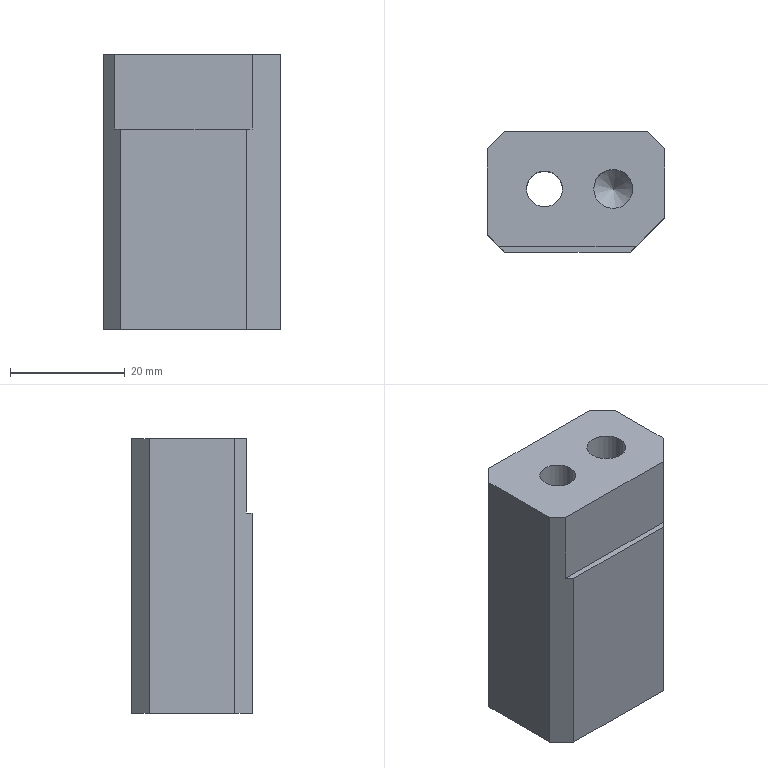Part | NX | features LIN_SOLID_COLOR 2 | 1 solid | 15 faces | box 31 x 21 x 48 mm | volume 26979 mm3 | plane 12 | cylinder 2 | cone 1 | commonest cylinder face diameters 6.28 x1 6.8 x1
STEP:
#1=CARTESIAN_POINT('',(657.878,13.865,1.5));
#2=VERTEX_POINT('',#1);
#3=CARTESIAN_POINT('',(655.878,15.865,1.5));
#4=VERTEX_POINT('',#3);
#5=CARTESIAN_POINT('',(655.878,15.865,1.5));
#6=DIRECTION('',(0.7071,-0.7071,0.));
#7=VECTOR('',#6,1000.);
#8=LINE('',#5,#7);
#9=EDGE_CURVE('',#2,#4,#8,.F.);
#10=ORIENTED_EDGE('',*,*,#9,.F.);
#11=CARTESIAN_POINT('',(681.878,13.865,1.5));
#12=VERTEX_POINT('',#11);
#13=CARTESIAN_POINT('',(305.33,13.865,1.5));
#14=DIRECTION('',(-1.,0.,0.));
#15=VECTOR('',#14,1000.);
#16=LINE('',#13,#15);
#17=EDGE_CURVE('',#12,#2,#16,.T.);
#18=ORIENTED_EDGE('',*,*,#17,.F.);
#19=CARTESIAN_POINT('',(686.878,18.865,1.5));
#20=VERTEX_POINT('',#19);
#21=CARTESIAN_POINT('',(686.878,18.865,1.5));
#22=DIRECTION('',(0.7071,0.7071,0.));
#23=VECTOR('',#22,1000.);
#24=LINE('',#21,#23);
#25=EDGE_CURVE('',#20,#12,#24,.F.);
#26=ORIENTED_EDGE('',*,*,#25,.F.);
#27=CARTESIAN_POINT('',(686.878,30.865,1.5));
#28=VERTEX_POINT('',#27);
#29=CARTESIAN_POINT('',(686.878,23.865,1.5));
#30=DIRECTION('',(0.,-1.,0.));
#31=VECTOR('',#30,1000.);
#32=LINE('',#29,#31);
#33=EDGE_CURVE('',#28,#20,#32,.T.);
#34=ORIENTED_EDGE('',*,*,#33,.F.);
#35=CARTESIAN_POINT('',(683.878,33.865,1.5));
#36=VERTEX_POINT('',#35);
#37=CARTESIAN_POINT('',(683.878,33.865,1.5));
#38=DIRECTION('',(-0.7071,0.7071,0.));
#39=VECTOR('',#38,1000.);
#40=LINE('',#37,#39);
#41=EDGE_CURVE('',#36,#28,#40,.F.);
#42=ORIENTED_EDGE('',*,*,#41,.F.);
#43=CARTESIAN_POINT('',(658.878,33.865,1.5));
#44=VERTEX_POINT('',#43);
#45=CARTESIAN_POINT('',(672.878,33.865,1.5));
#46=DIRECTION('',(1.,0.,0.));
#47=VECTOR('',#46,1000.);
#48=LINE('',#45,#47);
#49=EDGE_CURVE('',#44,#36,#48,.T.);
#50=ORIENTED_EDGE('',*,*,#49,.F.);
#51=CARTESIAN_POINT('',(655.878,30.865,1.5));
#52=VERTEX_POINT('',#51);
#53=CARTESIAN_POINT('',(658.878,33.865,1.5));
#54=DIRECTION('',(-0.7071,-0.7071,0.));
#55=VECTOR('',#54,1000.);
#56=LINE('',#53,#55);
#57=EDGE_CURVE('',#52,#44,#56,.F.);
#58=ORIENTED_EDGE('',*,*,#57,.F.);
#59=CARTESIAN_POINT('',(655.878,23.865,1.5));
#60=DIRECTION('',(0.,1.,0.));
#61=VECTOR('',#60,1000.);
#62=LINE('',#59,#61);
#63=EDGE_CURVE('',#4,#52,#62,.T.);
#64=ORIENTED_EDGE('',*,*,#63,.F.);
#65=EDGE_LOOP('',(#10,#18,#26,#34,#42,#50,#58,#64));
#66=FACE_BOUND('',#65,.T.);
#67=CARTESIAN_POINT('',(669.018,23.865,1.5));
#68=VERTEX_POINT('',#67);
#69=CARTESIAN_POINT('',(665.878,23.865,1.5));
#70=DIRECTION('',(0.,0.,1.));
#71=DIRECTION('',(1.,0.,0.));
#72=AXIS2_PLACEMENT_3D('',#69,#70,#71);
#73=CIRCLE('',#72,3.14);
#74=EDGE_CURVE('',#68,#68,#73,.F.);
#75=ORIENTED_EDGE('',*,*,#74,.T.);
#76=EDGE_LOOP('',(#75));
#77=FACE_BOUND('',#76,.T.);
#78=CARTESIAN_POINT('',(681.278,23.865,1.5));
#79=VERTEX_POINT('',#78);
#80=CARTESIAN_POINT('',(677.878,23.865,1.5));
#81=DIRECTION('',(0.,0.,-1.));
#82=DIRECTION('',(1.,0.,0.));
#83=AXIS2_PLACEMENT_3D('',#80,#81,#82);
#84=CIRCLE('',#83,3.4);
#85=EDGE_CURVE('',#79,#79,#84,.T.);
#86=ORIENTED_EDGE('',*,*,#85,.T.);
#87=EDGE_LOOP('',(#86));
#88=FACE_BOUND('',#87,.T.);
#89=CARTESIAN_POINT('',(305.33,343.366,1.5));
#90=DIRECTION('',(0.,0.,1.));
#91=DIRECTION('',(0.,-1.,0.));
#92=AXIS2_PLACEMENT_3D('',#89,#90,#91);
#93=PLANE('',#92);
#94=ADVANCED_FACE('',(#66,#77,#88),#93,.T.);
#95=CARTESIAN_POINT('',(658.878,12.865,-11.5));
#96=VERTEX_POINT('',#95);
#97=CARTESIAN_POINT('',(680.878,12.865,-11.5));
#98=VERTEX_POINT('',#97);
#99=CARTESIAN_POINT('',(672.878,12.865,-11.5));
#100=DIRECTION('',(1.,0.,0.));
#101=VECTOR('',#100,1000.);
#102=LINE('',#99,#101);
#103=EDGE_CURVE('',#96,#98,#102,.T.);
#104=ORIENTED_EDGE('',*,*,#103,.F.);
#105=CARTESIAN_POINT('',(658.878,12.865,-46.5));
#106=VERTEX_POINT('',#105);
#107=CARTESIAN_POINT('',(658.878,12.865,-28.49));
#108=DIRECTION('',(0.,0.,-1.));
#109=VECTOR('',#108,1000.);
#110=LINE('',#107,#109);
#111=EDGE_CURVE('',#96,#106,#110,.T.);
#112=ORIENTED_EDGE('',*,*,#111,.T.);
#113=CARTESIAN_POINT('',(680.878,12.865,-46.5));
#114=VERTEX_POINT('',#113);
#115=CARTESIAN_POINT('',(672.878,12.865,-46.5));
#116=DIRECTION('',(1.,0.,0.));
#117=VECTOR('',#116,1000.);
#118=LINE('',#115,#117);
#119=EDGE_CURVE('',#106,#114,#118,.T.);
#120=ORIENTED_EDGE('',*,*,#119,.T.);
#121=CARTESIAN_POINT('',(680.878,12.865,-28.49));
#122=DIRECTION('',(0.,0.,1.));
#123=VECTOR('',#122,1000.);
#124=LINE('',#121,#123);
#125=EDGE_CURVE('',#114,#98,#124,.T.);
#126=ORIENTED_EDGE('',*,*,#125,.T.);
#127=EDGE_LOOP('',(#104,#112,#120,#126));
#128=FACE_BOUND('',#127,.T.);
#129=CARTESIAN_POINT('',(672.878,12.865,-28.49));
#130=DIRECTION('',(0.,-1.,0.));
#131=DIRECTION('',(0.,0.,-1.));
#132=AXIS2_PLACEMENT_3D('',#129,#130,#131);
#133=PLANE('',#132);
#134=ADVANCED_FACE('',(#128),#133,.T.);
#135=CARTESIAN_POINT('',(655.878,15.865,-46.5));
#136=VERTEX_POINT('',#135);
#137=CARTESIAN_POINT('',(655.878,15.865,-28.49));
#138=DIRECTION('',(0.,0.,1.));
#139=VECTOR('',#138,1000.);
#140=LINE('',#137,#139);
#141=EDGE_CURVE('',#136,#4,#140,.T.);
#142=ORIENTED_EDGE('',*,*,#141,.T.);
#143=ORIENTED_EDGE('',*,*,#63,.T.);
#144=CARTESIAN_POINT('',(655.878,30.865,-46.5));
#145=VERTEX_POINT('',#144);
#146=CARTESIAN_POINT('',(655.878,30.865,-28.49));
#147=DIRECTION('',(0.,0.,-1.));
#148=VECTOR('',#147,1000.);
#149=LINE('',#146,#148);
#150=EDGE_CURVE('',#52,#145,#149,.T.);
#151=ORIENTED_EDGE('',*,*,#150,.T.);
#152=CARTESIAN_POINT('',(655.878,23.865,-46.5));
#153=DIRECTION('',(0.,-1.,0.));
#154=VECTOR('',#153,1000.);
#155=LINE('',#152,#154);
#156=EDGE_CURVE('',#145,#136,#155,.T.);
#157=ORIENTED_EDGE('',*,*,#156,.T.);
#158=EDGE_LOOP('',(#142,#143,#151,#157));
#159=FACE_BOUND('',#158,.T.);
#160=CARTESIAN_POINT('',(655.878,23.865,-28.49));
#161=DIRECTION('',(-1.,0.,0.));
#162=DIRECTION('',(0.,0.,1.));
#163=AXIS2_PLACEMENT_3D('',#160,#161,#162);
#164=PLANE('',#163);
#165=ADVANCED_FACE('',(#159),#164,.T.);
#166=ORIENTED_EDGE('',*,*,#49,.T.);
#167=CARTESIAN_POINT('',(683.878,33.865,-46.5));
#168=VERTEX_POINT('',#167);
#169=CARTESIAN_POINT('',(683.878,33.865,-28.49));
#170=DIRECTION('',(0.,0.,-1.));
#171=VECTOR('',#170,1000.);
#172=LINE('',#169,#171);
#173=EDGE_CURVE('',#36,#168,#172,.T.);
#174=ORIENTED_EDGE('',*,*,#173,.T.);
#175=CARTESIAN_POINT('',(658.878,33.865,-46.5));
#176=VERTEX_POINT('',#175);
#177=CARTESIAN_POINT('',(672.878,33.865,-46.5));
#178=DIRECTION('',(-1.,0.,0.));
#179=VECTOR('',#178,1000.);
#180=LINE('',#177,#179);
#181=EDGE_CURVE('',#168,#176,#180,.T.);
#182=ORIENTED_EDGE('',*,*,#181,.T.);
#183=CARTESIAN_POINT('',(658.878,33.865,-28.49));
#184=DIRECTION('',(0.,0.,1.));
#185=VECTOR('',#184,1000.);
#186=LINE('',#183,#185);
#187=EDGE_CURVE('',#176,#44,#186,.T.);
#188=ORIENTED_EDGE('',*,*,#187,.T.);
#189=EDGE_LOOP('',(#166,#174,#182,#188));
#190=FACE_BOUND('',#189,.T.);
#191=CARTESIAN_POINT('',(672.878,33.865,-28.49));
#192=DIRECTION('',(0.,1.,0.));
#193=DIRECTION('',(0.,0.,1.));
#194=AXIS2_PLACEMENT_3D('',#191,#192,#193);
#195=PLANE('',#194);
#196=ADVANCED_FACE('',(#190),#195,.T.);
#197=CARTESIAN_POINT('',(686.878,30.865,-46.5));
#198=VERTEX_POINT('',#197);
#199=CARTESIAN_POINT('',(686.878,30.865,-28.49));
#200=DIRECTION('',(0.,0.,1.));
#201=VECTOR('',#200,1000.);
#202=LINE('',#199,#201);
#203=EDGE_CURVE('',#198,#28,#202,.T.);
#204=ORIENTED_EDGE('',*,*,#203,.T.);
#205=ORIENTED_EDGE('',*,*,#33,.T.);
#206=CARTESIAN_POINT('',(686.878,18.865,-46.5));
#207=VERTEX_POINT('',#206);
#208=CARTESIAN_POINT('',(686.878,18.865,-28.49));
#209=DIRECTION('',(0.,0.,-1.));
#210=VECTOR('',#209,1000.);
#211=LINE('',#208,#210);
#212=EDGE_CURVE('',#20,#207,#211,.T.);
#213=ORIENTED_EDGE('',*,*,#212,.T.);
#214=CARTESIAN_POINT('',(686.878,23.865,-46.5));
#215=DIRECTION('',(0.,1.,0.));
#216=VECTOR('',#215,1000.);
#217=LINE('',#214,#216);
#218=EDGE_CURVE('',#207,#198,#217,.T.);
#219=ORIENTED_EDGE('',*,*,#218,.T.);
#220=EDGE_LOOP('',(#204,#205,#213,#219));
#221=FACE_BOUND('',#220,.T.);
#222=CARTESIAN_POINT('',(686.878,23.865,-28.49));
#223=DIRECTION('',(1.,0.,0.));
#224=DIRECTION('',(0.,0.,-1.));
#225=AXIS2_PLACEMENT_3D('',#222,#223,#224);
#226=PLANE('',#225);
#227=ADVANCED_FACE('',(#221),#226,.T.);
#228=CARTESIAN_POINT('',(669.018,23.865,-46.5));
#229=VERTEX_POINT('',#228);
#230=CARTESIAN_POINT('',(665.878,23.865,-46.5));
#231=DIRECTION('',(0.,0.,-1.));
#232=DIRECTION('',(1.,0.,0.));
#233=AXIS2_PLACEMENT_3D('',#230,#231,#232);
#234=CIRCLE('',#233,3.14);
#235=EDGE_CURVE('',#229,#229,#234,.T.);
#236=ORIENTED_EDGE('',*,*,#235,.T.);
#237=EDGE_LOOP('',(#236));
#238=FACE_BOUND('',#237,.T.);
#239=ORIENTED_EDGE('',*,*,#74,.F.);
#240=EDGE_LOOP('',(#239));
#241=FACE_BOUND('',#240,.T.);
#242=CARTESIAN_POINT('',(665.878,23.865,-63.49));
#243=DIRECTION('',(0.,0.,1.));
#244=DIRECTION('',(1.,0.,0.));
#245=AXIS2_PLACEMENT_3D('',#242,#243,#244);
#246=CYLINDRICAL_SURFACE('',#245,3.14);
#247=ADVANCED_FACE('',(#238,#241),#246,.F.);
#248=ORIENTED_EDGE('',*,*,#150,.F.);
#249=ORIENTED_EDGE('',*,*,#57,.T.);
#250=ORIENTED_EDGE('',*,*,#187,.F.);
#251=CARTESIAN_POINT('',(660.378,35.365,-46.5));
#252=DIRECTION('',(-0.7071,-0.7071,0.));
#253=VECTOR('',#252,1000.);
#254=LINE('',#251,#253);
#255=EDGE_CURVE('',#145,#176,#254,.F.);
#256=ORIENTED_EDGE('',*,*,#255,.F.);
#257=EDGE_LOOP('',(#248,#249,#250,#256));
#258=FACE_BOUND('',#257,.T.);
#259=CARTESIAN_POINT('',(658.878,33.865,-28.49));
#260=DIRECTION('',(0.7071,-0.7071,0.));
#261=DIRECTION('',(0.,0.,1.));
#262=AXIS2_PLACEMENT_3D('',#259,#260,#261);
#263=PLANE('',#262);
#264=ADVANCED_FACE('',(#258),#263,.F.);
#265=CARTESIAN_POINT('',(657.878,13.865,-11.5));
#266=VERTEX_POINT('',#265);
#267=CARTESIAN_POINT('',(655.878,15.865,-11.5));
#268=DIRECTION('',(-0.7071,0.7071,0.));
#269=VECTOR('',#268,1000.);
#270=LINE('',#267,#269);
#271=EDGE_CURVE('',#266,#96,#270,.F.);
#272=ORIENTED_EDGE('',*,*,#271,.F.);
#273=CARTESIAN_POINT('',(657.878,13.865,-28.49));
#274=DIRECTION('',(0.,0.,1.));
#275=VECTOR('',#274,1000.);
#276=LINE('',#273,#275);
#277=EDGE_CURVE('',#2,#266,#276,.F.);
#278=ORIENTED_EDGE('',*,*,#277,.F.);
#279=ORIENTED_EDGE('',*,*,#9,.T.);
#280=ORIENTED_EDGE('',*,*,#141,.F.);
#281=CARTESIAN_POINT('',(660.378,11.365,-46.5));
#282=DIRECTION('',(0.7071,-0.7071,0.));
#283=VECTOR('',#282,1000.);
#284=LINE('',#281,#283);
#285=EDGE_CURVE('',#106,#136,#284,.F.);
#286=ORIENTED_EDGE('',*,*,#285,.F.);
#287=ORIENTED_EDGE('',*,*,#111,.F.);
#288=EDGE_LOOP('',(#272,#278,#279,#280,#286,#287));
#289=FACE_BOUND('',#288,.T.);
#290=CARTESIAN_POINT('',(655.878,15.865,-28.49));
#291=DIRECTION('',(0.7071,0.7071,0.));
#292=DIRECTION('',(0.,0.,1.));
#293=AXIS2_PLACEMENT_3D('',#290,#291,#292);
#294=PLANE('',#293);
#295=ADVANCED_FACE('',(#289),#294,.F.);
#296=CARTESIAN_POINT('',(681.878,13.865,-11.5));
#297=VERTEX_POINT('',#296);
#298=CARTESIAN_POINT('',(686.878,18.865,-11.5));
#299=DIRECTION('',(-0.7071,-0.7071,0.));
#300=VECTOR('',#299,1000.);
#301=LINE('',#298,#300);
#302=EDGE_CURVE('',#98,#297,#301,.F.);
#303=ORIENTED_EDGE('',*,*,#302,.F.);
#304=ORIENTED_EDGE('',*,*,#125,.F.);
#305=CARTESIAN_POINT('',(678.878,10.865,-46.5));
#306=DIRECTION('',(0.7071,0.7071,0.));
#307=VECTOR('',#306,1000.);
#308=LINE('',#305,#307);
#309=EDGE_CURVE('',#207,#114,#308,.F.);
#310=ORIENTED_EDGE('',*,*,#309,.F.);
#311=ORIENTED_EDGE('',*,*,#212,.F.);
#312=ORIENTED_EDGE('',*,*,#25,.T.);
#313=CARTESIAN_POINT('',(681.878,13.865,-11.5));
#314=DIRECTION('',(0.,0.,1.));
#315=VECTOR('',#314,1000.);
#316=LINE('',#313,#315);
#317=EDGE_CURVE('',#12,#297,#316,.F.);
#318=ORIENTED_EDGE('',*,*,#317,.T.);
#319=EDGE_LOOP('',(#303,#304,#310,#311,#312,#318));
#320=FACE_BOUND('',#319,.T.);
#321=CARTESIAN_POINT('',(686.878,18.865,-28.49));
#322=DIRECTION('',(-0.7071,0.7071,0.));
#323=DIRECTION('',(0.,0.,-1.));
#324=AXIS2_PLACEMENT_3D('',#321,#322,#323);
#325=PLANE('',#324);
#326=ADVANCED_FACE('',(#320),#325,.F.);
#327=ORIENTED_EDGE('',*,*,#173,.F.);
#328=ORIENTED_EDGE('',*,*,#41,.T.);
#329=ORIENTED_EDGE('',*,*,#203,.F.);
#330=CARTESIAN_POINT('',(680.378,37.365,-46.5));
#331=DIRECTION('',(-0.7071,0.7071,0.));
#332=VECTOR('',#331,1000.);
#333=LINE('',#330,#332);
#334=EDGE_CURVE('',#168,#198,#333,.F.);
#335=ORIENTED_EDGE('',*,*,#334,.F.);
#336=EDGE_LOOP('',(#327,#328,#329,#335));
#337=FACE_BOUND('',#336,.T.);
#338=CARTESIAN_POINT('',(683.878,33.865,-28.49));
#339=DIRECTION('',(-0.7071,-0.7071,0.));
#340=DIRECTION('',(0.,0.,-1.));
#341=AXIS2_PLACEMENT_3D('',#338,#339,#340);
#342=PLANE('',#341);
#343=ADVANCED_FACE('',(#337),#342,.F.);
#344=ORIENTED_EDGE('',*,*,#181,.F.);
#345=ORIENTED_EDGE('',*,*,#334,.T.);
#346=ORIENTED_EDGE('',*,*,#218,.F.);
#347=ORIENTED_EDGE('',*,*,#309,.T.);
#348=ORIENTED_EDGE('',*,*,#119,.F.);
#349=ORIENTED_EDGE('',*,*,#285,.T.);
#350=ORIENTED_EDGE('',*,*,#156,.F.);
#351=ORIENTED_EDGE('',*,*,#255,.T.);
#352=EDGE_LOOP('',(#344,#345,#346,#347,#348,#349,#350,#351));
#353=FACE_BOUND('',#352,.T.);
#354=ORIENTED_EDGE('',*,*,#235,.F.);
#355=EDGE_LOOP('',(#354));
#356=FACE_BOUND('',#355,.T.);
#357=CARTESIAN_POINT('',(672.878,23.865,-46.5));
#358=DIRECTION('',(0.,0.,-1.));
#359=DIRECTION('',(-1.,0.,0.));
#360=AXIS2_PLACEMENT_3D('',#357,#358,#359);
#361=PLANE('',#360);
#362=ADVANCED_FACE('',(#353,#356),#361,.T.);
#363=CARTESIAN_POINT('',(674.478,23.865,-24.1));
#364=VERTEX_POINT('',#363);
#365=CARTESIAN_POINT('',(677.878,23.865,-24.1));
#366=DIRECTION('',(0.,0.,-1.));
#367=DIRECTION('',(-1.,0.,0.));
#368=AXIS2_PLACEMENT_3D('',#365,#366,#367);
#369=CIRCLE('',#368,3.4);
#370=EDGE_CURVE('',#364,#364,#369,.T.);
#371=ORIENTED_EDGE('',*,*,#370,.T.);
#372=EDGE_LOOP('',(#371));
#373=FACE_BOUND('',#372,.T.);
#374=ORIENTED_EDGE('',*,*,#85,.F.);
#375=EDGE_LOOP('',(#374));
#376=FACE_BOUND('',#375,.T.);
#377=CARTESIAN_POINT('',(677.878,23.865,1.5));
#378=DIRECTION('',(0.,0.,-1.));
#379=DIRECTION('',(1.,0.,0.));
#380=AXIS2_PLACEMENT_3D('',#377,#378,#379);
#381=CYLINDRICAL_SURFACE('',#380,3.4);
#382=ADVANCED_FACE('',(#373,#376),#381,.F.);
#383=CARTESIAN_POINT('',(677.878,23.865,-27.5));
#384=VERTEX_POINT('',#383);
#385=VERTEX_LOOP('',#384);
#386=FACE_BOUND('',#385,.T.);
#387=ORIENTED_EDGE('',*,*,#370,.F.);
#388=EDGE_LOOP('',(#387));
#389=FACE_BOUND('',#388,.T.);
#390=CARTESIAN_POINT('',(677.878,23.865,-24.1));
#391=DIRECTION('',(0.,0.,1.));
#392=DIRECTION('',(1.,0.,0.));
#393=AXIS2_PLACEMENT_3D('',#390,#391,#392);
#394=CONICAL_SURFACE('',#393,3.4,0.7854);
#395=ADVANCED_FACE('',(#386,#389),#394,.F.);
#396=ORIENTED_EDGE('',*,*,#271,.T.);
#397=ORIENTED_EDGE('',*,*,#103,.T.);
#398=ORIENTED_EDGE('',*,*,#302,.T.);
#399=CARTESIAN_POINT('',(671.378,13.865,-11.5));
#400=DIRECTION('',(1.,0.,0.));
#401=VECTOR('',#400,1000.);
#402=LINE('',#399,#401);
#403=EDGE_CURVE('',#297,#266,#402,.F.);
#404=ORIENTED_EDGE('',*,*,#403,.T.);
#405=EDGE_LOOP('',(#396,#397,#398,#404));
#406=FACE_BOUND('',#405,.T.);
#407=CARTESIAN_POINT('',(671.378,5.865,-11.5));
#408=DIRECTION('',(0.,0.,-1.));
#409=DIRECTION('',(0.,1.,0.));
#410=AXIS2_PLACEMENT_3D('',#407,#408,#409);
#411=PLANE('',#410);
#412=ADVANCED_FACE('',(#406),#411,.F.);
#413=ORIENTED_EDGE('',*,*,#17,.T.);
#414=ORIENTED_EDGE('',*,*,#277,.T.);
#415=ORIENTED_EDGE('',*,*,#403,.F.);
#416=ORIENTED_EDGE('',*,*,#317,.F.);
#417=EDGE_LOOP('',(#413,#414,#415,#416));
#418=FACE_BOUND('',#417,.T.);
#419=CARTESIAN_POINT('',(671.378,13.865,-11.5));
#420=DIRECTION('',(0.,1.,0.));
#421=DIRECTION('',(0.,0.,1.));
#422=AXIS2_PLACEMENT_3D('',#419,#420,#421);
#423=PLANE('',#422);
#424=ADVANCED_FACE('',(#418),#423,.F.);
#425=CLOSED_SHELL('',(#94,#134,#165,#196,#227,#247,#264,#295,#326,#343,#362,#382,#395,#412,#424));
#426=MANIFOLD_SOLID_BREP('',#425);
#427=(LENGTH_UNIT()NAMED_UNIT(*)SI_UNIT(.MILLI.,.METRE.));
#428=UNCERTAINTY_MEASURE_WITH_UNIT(LENGTH_MEASURE(0.00001),#427,'','');
#429=(NAMED_UNIT(*)PLANE_ANGLE_UNIT()SI_UNIT($,.RADIAN.));
#430=(NAMED_UNIT(*)SI_UNIT($,.STERADIAN.)SOLID_ANGLE_UNIT());
#431=(GEOMETRIC_REPRESENTATION_CONTEXT(3)GLOBAL_UNCERTAINTY_ASSIGNED_CONTEXT((#428))GLOBAL_UNIT_ASSIGNED_CONTEXT((#427,#429,#430))REPRESENTATION_CONTEXT('',''));
#432=ADVANCED_BREP_SHAPE_REPRESENTATION('',(#426),#431);